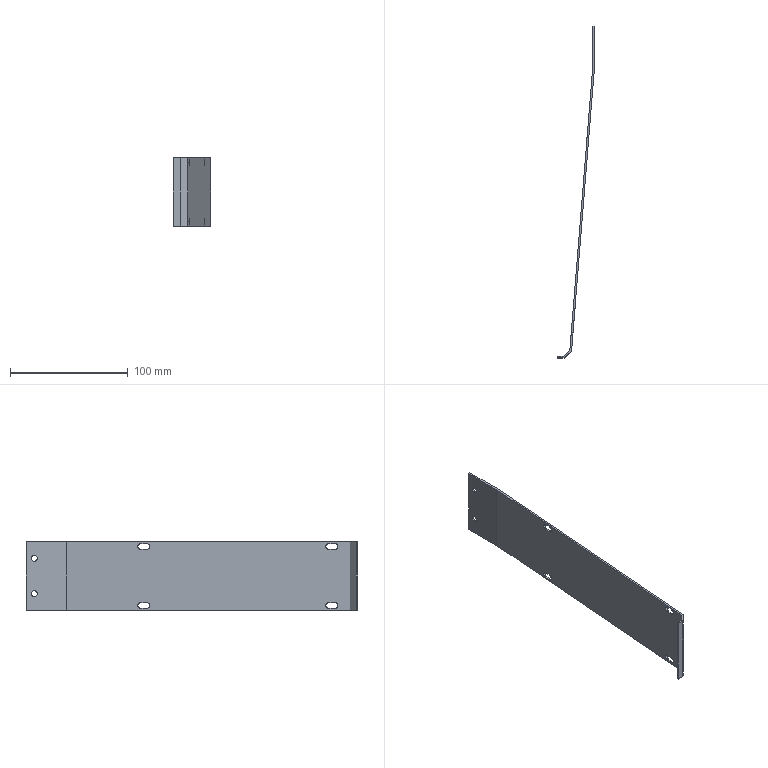Part | SolidWorks | features ICE 2, ExtruThin 1, MirrorPattern 1 | 1 solid | 36 faces | box 31.5 x 281.5 x 58 mm | volume 24856 mm3 | plane 20 | cylinder 16 | commonest cylinder face diameters 5 x16
STEP:
#1=CARTESIAN_POINT('',(-18.024,-256.762,6.5));
#2=VERTEX_POINT('',#1);
#3=CARTESIAN_POINT('',(-17.823,-254.27,4.));
#4=VERTEX_POINT('',#3);
#5=CARTESIAN_POINT('',(-18.024,-256.762,4.));
#6=DIRECTION('',(-0.9967,0.08065,0.));
#7=DIRECTION('',(0.08065,0.9967,0.));
#8=AXIS2_PLACEMENT_3D('',#5,#6,#7);
#9=CIRCLE('',#8,2.5);
#10=EDGE_CURVE('',#2,#4,#9,.T.);
#11=ORIENTED_EDGE('',*,*,#10,.T.);
#12=CARTESIAN_POINT('',(-16.328,-254.391,4.));
#13=VERTEX_POINT('',#12);
#14=CARTESIAN_POINT('',(-26.295,-253.584,4.));
#15=DIRECTION('',(0.9967,-0.08065,0.));
#16=VECTOR('',#15,1000.);
#17=LINE('',#14,#16);
#18=EDGE_CURVE('',#4,#13,#17,.T.);
#19=ORIENTED_EDGE('',*,*,#18,.T.);
#20=CARTESIAN_POINT('',(-16.529,-256.883,6.5));
#21=VERTEX_POINT('',#20);
#22=CARTESIAN_POINT('',(-16.529,-256.883,4.));
#23=DIRECTION('',(-0.9967,0.08065,0.));
#24=DIRECTION('',(-0.08065,-0.9967,0.));
#25=AXIS2_PLACEMENT_3D('',#22,#23,#24);
#26=CIRCLE('',#25,2.5);
#27=EDGE_CURVE('',#21,#13,#26,.T.);
#28=ORIENTED_EDGE('',*,*,#27,.F.);
#29=CARTESIAN_POINT('',(-26.497,-256.076,6.5));
#30=DIRECTION('',(0.9967,-0.08065,0.));
#31=VECTOR('',#30,1000.);
#32=LINE('',#29,#31);
#33=EDGE_CURVE('',#2,#21,#32,.T.);
#34=ORIENTED_EDGE('',*,*,#33,.F.);
#35=EDGE_LOOP('',(#11,#19,#28,#34));
#36=FACE_OUTER_BOUND('',#35,.T.);
#37=CARTESIAN_POINT('',(-26.497,-256.076,4.));
#38=DIRECTION('',(0.9967,-0.08065,0.));
#39=DIRECTION('',(0.08065,0.9967,0.));
#40=AXIS2_PLACEMENT_3D('',#37,#38,#39);
#41=CYLINDRICAL_SURFACE('',#40,2.5);
#42=ADVANCED_FACE('',(#36),#41,.F.);
#43=CARTESIAN_POINT('',(-5.12,-97.283,6.5));
#44=VERTEX_POINT('',#43);
#45=CARTESIAN_POINT('',(-4.919,-94.791,4.));
#46=VERTEX_POINT('',#45);
#47=CARTESIAN_POINT('',(-5.12,-97.283,4.));
#48=DIRECTION('',(-0.9967,0.08065,0.));
#49=DIRECTION('',(0.08065,0.9967,0.));
#50=AXIS2_PLACEMENT_3D('',#47,#48,#49);
#51=CIRCLE('',#50,2.5);
#52=EDGE_CURVE('',#44,#46,#51,.T.);
#53=ORIENTED_EDGE('',*,*,#52,.T.);
#54=CARTESIAN_POINT('',(-3.424,-94.912,4.));
#55=VERTEX_POINT('',#54);
#56=CARTESIAN_POINT('',(-13.391,-94.106,4.));
#57=DIRECTION('',(0.9967,-0.08065,0.));
#58=VECTOR('',#57,1000.);
#59=LINE('',#56,#58);
#60=EDGE_CURVE('',#46,#55,#59,.T.);
#61=ORIENTED_EDGE('',*,*,#60,.T.);
#62=CARTESIAN_POINT('',(-3.625,-97.404,6.5));
#63=VERTEX_POINT('',#62);
#64=CARTESIAN_POINT('',(-3.625,-97.404,4.));
#65=DIRECTION('',(-0.9967,0.08065,0.));
#66=DIRECTION('',(0.08065,0.9967,0.));
#67=AXIS2_PLACEMENT_3D('',#64,#65,#66);
#68=CIRCLE('',#67,2.5);
#69=EDGE_CURVE('',#63,#55,#68,.T.);
#70=ORIENTED_EDGE('',*,*,#69,.F.);
#71=CARTESIAN_POINT('',(-13.593,-96.597,6.5));
#72=DIRECTION('',(0.9967,-0.08065,0.));
#73=VECTOR('',#72,1000.);
#74=LINE('',#71,#73);
#75=EDGE_CURVE('',#44,#63,#74,.T.);
#76=ORIENTED_EDGE('',*,*,#75,.F.);
#77=EDGE_LOOP('',(#53,#61,#70,#76));
#78=FACE_OUTER_BOUND('',#77,.T.);
#79=CARTESIAN_POINT('',(-13.593,-96.597,4.));
#80=DIRECTION('',(0.9967,-0.08065,0.));
#81=DIRECTION('',(0.08065,0.9967,0.));
#82=AXIS2_PLACEMENT_3D('',#79,#80,#81);
#83=CYLINDRICAL_SURFACE('',#82,2.5);
#84=ADVANCED_FACE('',(#78),#83,.F.);
#85=CARTESIAN_POINT('',(-17.823,-254.27,54.));
#86=VERTEX_POINT('',#85);
#87=CARTESIAN_POINT('',(-18.024,-256.762,56.5));
#88=VERTEX_POINT('',#87);
#89=CARTESIAN_POINT('',(-18.024,-256.762,54.));
#90=DIRECTION('',(0.9967,-0.08065,0.));
#91=DIRECTION('',(0.08065,0.9967,0.));
#92=AXIS2_PLACEMENT_3D('',#89,#90,#91);
#93=CIRCLE('',#92,2.5);
#94=EDGE_CURVE('',#86,#88,#93,.T.);
#95=ORIENTED_EDGE('',*,*,#94,.F.);
#96=CARTESIAN_POINT('',(-16.328,-254.391,54.));
#97=VERTEX_POINT('',#96);
#98=CARTESIAN_POINT('',(-26.295,-253.584,54.));
#99=DIRECTION('',(0.9967,-0.08065,0.));
#100=VECTOR('',#99,1000.);
#101=LINE('',#98,#100);
#102=EDGE_CURVE('',#86,#97,#101,.T.);
#103=ORIENTED_EDGE('',*,*,#102,.T.);
#104=CARTESIAN_POINT('',(-16.529,-256.883,56.5));
#105=VERTEX_POINT('',#104);
#106=CARTESIAN_POINT('',(-16.529,-256.883,54.));
#107=DIRECTION('',(0.9967,-0.08065,0.));
#108=DIRECTION('',(-0.08065,-0.9967,0.));
#109=AXIS2_PLACEMENT_3D('',#106,#107,#108);
#110=CIRCLE('',#109,2.5);
#111=EDGE_CURVE('',#97,#105,#110,.T.);
#112=ORIENTED_EDGE('',*,*,#111,.T.);
#113=CARTESIAN_POINT('',(-26.497,-256.076,56.5));
#114=DIRECTION('',(0.9967,-0.08065,0.));
#115=VECTOR('',#114,1000.);
#116=LINE('',#113,#115);
#117=EDGE_CURVE('',#88,#105,#116,.T.);
#118=ORIENTED_EDGE('',*,*,#117,.F.);
#119=EDGE_LOOP('',(#95,#103,#112,#118));
#120=FACE_OUTER_BOUND('',#119,.T.);
#121=CARTESIAN_POINT('',(-26.497,-256.076,54.));
#122=DIRECTION('',(0.9967,-0.08065,0.));
#123=DIRECTION('',(0.08065,0.9967,0.));
#124=AXIS2_PLACEMENT_3D('',#121,#122,#123);
#125=CYLINDRICAL_SURFACE('',#124,2.5);
#126=ADVANCED_FACE('',(#120),#125,.F.);
#127=CARTESIAN_POINT('',(-4.919,-94.791,54.));
#128=VERTEX_POINT('',#127);
#129=CARTESIAN_POINT('',(-5.12,-97.283,56.5));
#130=VERTEX_POINT('',#129);
#131=CARTESIAN_POINT('',(-5.12,-97.283,54.));
#132=DIRECTION('',(0.9967,-0.08065,0.));
#133=DIRECTION('',(0.08065,0.9967,0.));
#134=AXIS2_PLACEMENT_3D('',#131,#132,#133);
#135=CIRCLE('',#134,2.5);
#136=EDGE_CURVE('',#128,#130,#135,.T.);
#137=ORIENTED_EDGE('',*,*,#136,.F.);
#138=CARTESIAN_POINT('',(-3.424,-94.912,54.));
#139=VERTEX_POINT('',#138);
#140=CARTESIAN_POINT('',(-13.391,-94.106,54.));
#141=DIRECTION('',(0.9967,-0.08065,0.));
#142=VECTOR('',#141,1000.);
#143=LINE('',#140,#142);
#144=EDGE_CURVE('',#128,#139,#143,.T.);
#145=ORIENTED_EDGE('',*,*,#144,.T.);
#146=CARTESIAN_POINT('',(-3.625,-97.404,56.5));
#147=VERTEX_POINT('',#146);
#148=CARTESIAN_POINT('',(-3.625,-97.404,54.));
#149=DIRECTION('',(0.9967,-0.08065,0.));
#150=DIRECTION('',(0.08065,0.9967,0.));
#151=AXIS2_PLACEMENT_3D('',#148,#149,#150);
#152=CIRCLE('',#151,2.5);
#153=EDGE_CURVE('',#139,#147,#152,.T.);
#154=ORIENTED_EDGE('',*,*,#153,.T.);
#155=CARTESIAN_POINT('',(-13.593,-96.597,56.5));
#156=DIRECTION('',(0.9967,-0.08065,0.));
#157=VECTOR('',#156,1000.);
#158=LINE('',#155,#157);
#159=EDGE_CURVE('',#130,#147,#158,.T.);
#160=ORIENTED_EDGE('',*,*,#159,.F.);
#161=EDGE_LOOP('',(#137,#145,#154,#160));
#162=FACE_OUTER_BOUND('',#161,.T.);
#163=CARTESIAN_POINT('',(-13.593,-96.597,54.));
#164=DIRECTION('',(0.9967,-0.08065,0.));
#165=DIRECTION('',(0.08065,0.9967,0.));
#166=AXIS2_PLACEMENT_3D('',#163,#164,#165);
#167=CYLINDRICAL_SURFACE('',#166,2.5);
#168=ADVANCED_FACE('',(#162),#167,.F.);
#169=CARTESIAN_POINT('',(0.,-9.5,44.));
#170=VERTEX_POINT('',#169);
#171=CARTESIAN_POINT('',(0.,-4.5,44.));
#172=VERTEX_POINT('',#171);
#173=CARTESIAN_POINT('',(0.,-7.,44.));
#174=DIRECTION('',(1.,0.,0.));
#175=DIRECTION('',(0.,1.,0.));
#176=AXIS2_PLACEMENT_3D('',#173,#174,#175);
#177=CIRCLE('',#176,2.5);
#178=EDGE_CURVE('',#170,#172,#177,.T.);
#179=ORIENTED_EDGE('',*,*,#178,.F.);
#180=CARTESIAN_POINT('',(1.5,-9.5,44.));
#181=VERTEX_POINT('',#180);
#182=CARTESIAN_POINT('',(-8.5,-9.5,44.));
#183=DIRECTION('',(1.,0.,0.));
#184=VECTOR('',#183,1000.);
#185=LINE('',#182,#184);
#186=EDGE_CURVE('',#170,#181,#185,.T.);
#187=ORIENTED_EDGE('',*,*,#186,.T.);
#188=CARTESIAN_POINT('',(1.5,-4.5,44.));
#189=VERTEX_POINT('',#188);
#190=CARTESIAN_POINT('',(1.5,-7.,44.));
#191=DIRECTION('',(1.,0.,0.));
#192=DIRECTION('',(0.,1.,0.));
#193=AXIS2_PLACEMENT_3D('',#190,#191,#192);
#194=CIRCLE('',#193,2.5);
#195=EDGE_CURVE('',#181,#189,#194,.T.);
#196=ORIENTED_EDGE('',*,*,#195,.T.);
#197=CARTESIAN_POINT('',(-8.5,-4.5,44.));
#198=DIRECTION('',(1.,0.,0.));
#199=VECTOR('',#198,1000.);
#200=LINE('',#197,#199);
#201=EDGE_CURVE('',#172,#189,#200,.T.);
#202=ORIENTED_EDGE('',*,*,#201,.F.);
#203=EDGE_LOOP('',(#179,#187,#196,#202));
#204=FACE_OUTER_BOUND('',#203,.T.);
#205=CARTESIAN_POINT('',(-8.5,-7.,44.));
#206=DIRECTION('',(1.,0.,0.));
#207=DIRECTION('',(0.,1.,0.));
#208=AXIS2_PLACEMENT_3D('',#205,#206,#207);
#209=CYLINDRICAL_SURFACE('',#208,2.5);
#210=ADVANCED_FACE('',(#204),#209,.F.);
#211=CARTESIAN_POINT('',(0.,-9.5,14.));
#212=VERTEX_POINT('',#211);
#213=CARTESIAN_POINT('',(0.,-4.5,14.));
#214=VERTEX_POINT('',#213);
#215=CARTESIAN_POINT('',(0.,-7.,14.));
#216=DIRECTION('',(1.,0.,0.));
#217=DIRECTION('',(0.,1.,0.));
#218=AXIS2_PLACEMENT_3D('',#215,#216,#217);
#219=CIRCLE('',#218,2.5);
#220=EDGE_CURVE('',#212,#214,#219,.T.);
#221=ORIENTED_EDGE('',*,*,#220,.F.);
#222=CARTESIAN_POINT('',(1.5,-9.5,14.));
#223=VERTEX_POINT('',#222);
#224=CARTESIAN_POINT('',(-8.5,-9.5,14.));
#225=DIRECTION('',(1.,0.,0.));
#226=VECTOR('',#225,1000.);
#227=LINE('',#224,#226);
#228=EDGE_CURVE('',#212,#223,#227,.T.);
#229=ORIENTED_EDGE('',*,*,#228,.T.);
#230=CARTESIAN_POINT('',(1.5,-4.5,14.));
#231=VERTEX_POINT('',#230);
#232=CARTESIAN_POINT('',(1.5,-7.,14.));
#233=DIRECTION('',(1.,0.,0.));
#234=DIRECTION('',(0.,1.,0.));
#235=AXIS2_PLACEMENT_3D('',#232,#233,#234);
#236=CIRCLE('',#235,2.5);
#237=EDGE_CURVE('',#223,#231,#236,.T.);
#238=ORIENTED_EDGE('',*,*,#237,.T.);
#239=CARTESIAN_POINT('',(-8.5,-4.5,14.));
#240=DIRECTION('',(1.,0.,0.));
#241=VECTOR('',#240,1000.);
#242=LINE('',#239,#241);
#243=EDGE_CURVE('',#214,#231,#242,.T.);
#244=ORIENTED_EDGE('',*,*,#243,.F.);
#245=EDGE_LOOP('',(#221,#229,#238,#244));
#246=FACE_OUTER_BOUND('',#245,.T.);
#247=CARTESIAN_POINT('',(-8.5,-7.,14.));
#248=DIRECTION('',(1.,0.,0.));
#249=DIRECTION('',(0.,1.,0.));
#250=AXIS2_PLACEMENT_3D('',#247,#248,#249);
#251=CYLINDRICAL_SURFACE('',#250,2.5);
#252=ADVANCED_FACE('',(#246),#251,.F.);
#253=CARTESIAN_POINT('',(-4.029,-102.388,6.5));
#254=VERTEX_POINT('',#253);
#255=CARTESIAN_POINT('',(-3.625,-97.404,6.5));
#256=DIRECTION('',(0.08065,0.9967,0.));
#257=VECTOR('',#256,1000.);
#258=LINE('',#255,#257);
#259=EDGE_CURVE('',#254,#63,#258,.T.);
#260=ORIENTED_EDGE('',*,*,#259,.T.);
#261=ORIENTED_EDGE('',*,*,#69,.T.);
#262=CARTESIAN_POINT('',(-3.625,-97.404,1.5));
#263=VERTEX_POINT('',#262);
#264=CARTESIAN_POINT('',(-3.625,-97.404,4.));
#265=DIRECTION('',(-0.9967,0.08065,0.));
#266=DIRECTION('',(0.08065,0.9967,0.));
#267=AXIS2_PLACEMENT_3D('',#264,#265,#266);
#268=CIRCLE('',#267,2.5);
#269=EDGE_CURVE('',#55,#263,#268,.T.);
#270=ORIENTED_EDGE('',*,*,#269,.T.);
#271=CARTESIAN_POINT('',(-4.029,-102.388,1.5));
#272=VERTEX_POINT('',#271);
#273=CARTESIAN_POINT('',(-3.625,-97.404,1.5));
#274=DIRECTION('',(-0.08065,-0.9967,0.));
#275=VECTOR('',#274,1000.);
#276=LINE('',#273,#275);
#277=EDGE_CURVE('',#263,#272,#276,.T.);
#278=ORIENTED_EDGE('',*,*,#277,.T.);
#279=CARTESIAN_POINT('',(-4.029,-102.388,4.));
#280=DIRECTION('',(-0.9967,0.08065,0.));
#281=DIRECTION('',(0.08065,0.9967,0.));
#282=AXIS2_PLACEMENT_3D('',#279,#280,#281);
#283=CIRCLE('',#282,2.5);
#284=EDGE_CURVE('',#272,#254,#283,.T.);
#285=ORIENTED_EDGE('',*,*,#284,.T.);
#286=EDGE_LOOP('',(#260,#261,#270,#278,#285));
#287=FACE_BOUND('',#286,.T.);
#288=CARTESIAN_POINT('',(-16.932,-261.866,56.5));
#289=VERTEX_POINT('',#288);
#290=CARTESIAN_POINT('',(-16.932,-261.866,51.5));
#291=VERTEX_POINT('',#290);
#292=CARTESIAN_POINT('',(-16.932,-261.866,54.));
#293=DIRECTION('',(0.9967,-0.08065,0.));
#294=DIRECTION('',(-0.08065,-0.9967,0.));
#295=AXIS2_PLACEMENT_3D('',#292,#293,#294);
#296=CIRCLE('',#295,2.5);
#297=EDGE_CURVE('',#289,#291,#296,.T.);
#298=ORIENTED_EDGE('',*,*,#297,.F.);
#299=CARTESIAN_POINT('',(-16.932,-261.866,56.5));
#300=DIRECTION('',(-0.08065,-0.9967,0.));
#301=VECTOR('',#300,1000.);
#302=LINE('',#299,#301);
#303=EDGE_CURVE('',#105,#289,#302,.T.);
#304=ORIENTED_EDGE('',*,*,#303,.F.);
#305=ORIENTED_EDGE('',*,*,#111,.F.);
#306=CARTESIAN_POINT('',(-16.529,-256.883,51.5));
#307=VERTEX_POINT('',#306);
#308=CARTESIAN_POINT('',(-16.529,-256.883,54.));
#309=DIRECTION('',(0.9967,-0.08065,0.));
#310=DIRECTION('',(-0.08065,-0.9967,0.));
#311=AXIS2_PLACEMENT_3D('',#308,#309,#310);
#312=CIRCLE('',#311,2.5);
#313=EDGE_CURVE('',#307,#97,#312,.T.);
#314=ORIENTED_EDGE('',*,*,#313,.F.);
#315=CARTESIAN_POINT('',(-16.932,-261.866,51.5));
#316=DIRECTION('',(0.08065,0.9967,0.));
#317=VECTOR('',#316,1000.);
#318=LINE('',#315,#317);
#319=EDGE_CURVE('',#291,#307,#318,.T.);
#320=ORIENTED_EDGE('',*,*,#319,.F.);
#321=EDGE_LOOP('',(#298,#304,#305,#314,#320));
#322=FACE_BOUND('',#321,.T.);
#323=CARTESIAN_POINT('',(-3.625,-97.404,51.5));
#324=VERTEX_POINT('',#323);
#325=CARTESIAN_POINT('',(-3.625,-97.404,54.));
#326=DIRECTION('',(0.9967,-0.08065,0.));
#327=DIRECTION('',(0.08065,0.9967,0.));
#328=AXIS2_PLACEMENT_3D('',#325,#326,#327);
#329=CIRCLE('',#328,2.5);
#330=EDGE_CURVE('',#324,#139,#329,.T.);
#331=ORIENTED_EDGE('',*,*,#330,.F.);
#332=CARTESIAN_POINT('',(-4.029,-102.388,51.5));
#333=VERTEX_POINT('',#332);
#334=CARTESIAN_POINT('',(-3.625,-97.404,51.5));
#335=DIRECTION('',(0.08065,0.9967,0.));
#336=VECTOR('',#335,1000.);
#337=LINE('',#334,#336);
#338=EDGE_CURVE('',#333,#324,#337,.T.);
#339=ORIENTED_EDGE('',*,*,#338,.F.);
#340=CARTESIAN_POINT('',(-4.029,-102.388,56.5));
#341=VERTEX_POINT('',#340);
#342=CARTESIAN_POINT('',(-4.029,-102.388,54.));
#343=DIRECTION('',(0.9967,-0.08065,0.));
#344=DIRECTION('',(0.08065,0.9967,0.));
#345=AXIS2_PLACEMENT_3D('',#342,#343,#344);
#346=CIRCLE('',#345,2.5);
#347=EDGE_CURVE('',#341,#333,#346,.T.);
#348=ORIENTED_EDGE('',*,*,#347,.F.);
#349=CARTESIAN_POINT('',(-3.625,-97.404,56.5));
#350=DIRECTION('',(-0.08065,-0.9967,0.));
#351=VECTOR('',#350,1000.);
#352=LINE('',#349,#351);
#353=EDGE_CURVE('',#147,#341,#352,.T.);
#354=ORIENTED_EDGE('',*,*,#353,.F.);
#355=ORIENTED_EDGE('',*,*,#153,.F.);
#356=EDGE_LOOP('',(#331,#339,#348,#354,#355));
#357=FACE_BOUND('',#356,.T.);
#358=CARTESIAN_POINT('',(1.5,-34.061,0.));
#359=VERTEX_POINT('',#358);
#360=CARTESIAN_POINT('',(-18.053,-275.711,0.));
#361=VERTEX_POINT('',#360);
#362=CARTESIAN_POINT('',(1.495,-34.121,0.));
#363=DIRECTION('',(-0.08065,-0.9967,0.));
#364=VECTOR('',#363,1000.);
#365=LINE('',#362,#364);
#366=EDGE_CURVE('',#359,#361,#365,.T.);
#367=ORIENTED_EDGE('',*,*,#366,.F.);
#368=CARTESIAN_POINT('',(1.5,-34.061,58.));
#369=VERTEX_POINT('',#368);
#370=CARTESIAN_POINT('',(1.5,-34.061,58.));
#371=DIRECTION('',(0.,0.,-1.));
#372=VECTOR('',#371,1000.);
#373=LINE('',#370,#372);
#374=EDGE_CURVE('',#369,#359,#373,.T.);
#375=ORIENTED_EDGE('',*,*,#374,.F.);
#376=CARTESIAN_POINT('',(-18.053,-275.711,58.));
#377=VERTEX_POINT('',#376);
#378=CARTESIAN_POINT('',(1.495,-34.121,58.));
#379=DIRECTION('',(-0.08065,-0.9967,0.));
#380=VECTOR('',#379,1000.);
#381=LINE('',#378,#380);
#382=EDGE_CURVE('',#369,#377,#381,.T.);
#383=ORIENTED_EDGE('',*,*,#382,.T.);
#384=CARTESIAN_POINT('',(-18.053,-275.711,58.));
#385=DIRECTION('',(0.,0.,-1.));
#386=VECTOR('',#385,1000.);
#387=LINE('',#384,#386);
#388=EDGE_CURVE('',#377,#361,#387,.T.);
#389=ORIENTED_EDGE('',*,*,#388,.T.);
#390=EDGE_LOOP('',(#367,#375,#383,#389));
#391=FACE_OUTER_BOUND('',#390,.T.);
#392=CARTESIAN_POINT('',(-16.529,-256.883,1.5));
#393=VERTEX_POINT('',#392);
#394=CARTESIAN_POINT('',(-16.932,-261.866,1.5));
#395=VERTEX_POINT('',#394);
#396=CARTESIAN_POINT('',(-16.932,-261.866,1.5));
#397=DIRECTION('',(-0.08065,-0.9967,0.));
#398=VECTOR('',#397,1000.);
#399=LINE('',#396,#398);
#400=EDGE_CURVE('',#393,#395,#399,.T.);
#401=ORIENTED_EDGE('',*,*,#400,.T.);
#402=CARTESIAN_POINT('',(-16.932,-261.866,6.5));
#403=VERTEX_POINT('',#402);
#404=CARTESIAN_POINT('',(-16.932,-261.866,4.));
#405=DIRECTION('',(-0.9967,0.08065,0.));
#406=DIRECTION('',(-0.08065,-0.9967,0.));
#407=AXIS2_PLACEMENT_3D('',#404,#405,#406);
#408=CIRCLE('',#407,2.5);
#409=EDGE_CURVE('',#395,#403,#408,.T.);
#410=ORIENTED_EDGE('',*,*,#409,.T.);
#411=CARTESIAN_POINT('',(-16.932,-261.866,6.5));
#412=DIRECTION('',(0.08065,0.9967,0.));
#413=VECTOR('',#412,1000.);
#414=LINE('',#411,#413);
#415=EDGE_CURVE('',#403,#21,#414,.T.);
#416=ORIENTED_EDGE('',*,*,#415,.T.);
#417=ORIENTED_EDGE('',*,*,#27,.T.);
#418=CARTESIAN_POINT('',(-16.529,-256.883,4.));
#419=DIRECTION('',(-0.9967,0.08065,0.));
#420=DIRECTION('',(-0.08065,-0.9967,0.));
#421=AXIS2_PLACEMENT_3D('',#418,#419,#420);
#422=CIRCLE('',#421,2.5);
#423=EDGE_CURVE('',#13,#393,#422,.T.);
#424=ORIENTED_EDGE('',*,*,#423,.T.);
#425=EDGE_LOOP('',(#401,#410,#416,#417,#424));
#426=FACE_BOUND('',#425,.T.);
#427=CARTESIAN_POINT('',(1.495,-34.121,58.));
#428=DIRECTION('',(0.9967,-0.08065,0.));
#429=DIRECTION('',(0.08065,0.9967,0.));
#430=AXIS2_PLACEMENT_3D('',#427,#428,#429);
#431=PLANE('',#430);
#432=ADVANCED_FACE('',(#287,#322,#357,#391,#426),#431,.T.);
#433=ORIENTED_EDGE('',*,*,#52,.F.);
#434=CARTESIAN_POINT('',(-5.524,-102.267,6.5));
#435=VERTEX_POINT('',#434);
#436=CARTESIAN_POINT('',(0.,-34.,6.5));
#437=DIRECTION('',(0.08065,0.9967,0.));
#438=VECTOR('',#437,1000.);
#439=LINE('',#436,#438);
#440=EDGE_CURVE('',#435,#44,#439,.T.);
#441=ORIENTED_EDGE('',*,*,#440,.F.);
#442=CARTESIAN_POINT('',(-5.524,-102.267,1.5));
#443=VERTEX_POINT('',#442);
#444=CARTESIAN_POINT('',(-5.524,-102.267,4.));
#445=DIRECTION('',(-0.9967,0.08065,0.));
#446=DIRECTION('',(0.08065,0.9967,0.));
#447=AXIS2_PLACEMENT_3D('',#444,#445,#446);
#448=CIRCLE('',#447,2.5);
#449=EDGE_CURVE('',#443,#435,#448,.T.);
#450=ORIENTED_EDGE('',*,*,#449,.F.);
#451=CARTESIAN_POINT('',(-5.12,-97.283,1.5));
#452=VERTEX_POINT('',#451);
#453=CARTESIAN_POINT('',(0.,-34.,1.5));
#454=DIRECTION('',(-0.08065,-0.9967,0.));
#455=VECTOR('',#454,1000.);
#456=LINE('',#453,#455);
#457=EDGE_CURVE('',#452,#443,#456,.T.);
#458=ORIENTED_EDGE('',*,*,#457,.F.);
#459=CARTESIAN_POINT('',(-5.12,-97.283,4.));
#460=DIRECTION('',(-0.9967,0.08065,0.));
#461=DIRECTION('',(0.08065,0.9967,0.));
#462=AXIS2_PLACEMENT_3D('',#459,#460,#461);
#463=CIRCLE('',#462,2.5);
#464=EDGE_CURVE('',#46,#452,#463,.T.);
#465=ORIENTED_EDGE('',*,*,#464,.F.);
#466=EDGE_LOOP('',(#433,#441,#450,#458,#465));
#467=FACE_BOUND('',#466,.T.);
#468=CARTESIAN_POINT('',(-18.428,-261.745,56.5));
#469=VERTEX_POINT('',#468);
#470=CARTESIAN_POINT('',(0.,-34.,56.5));
#471=DIRECTION('',(-0.08065,-0.9967,0.));
#472=VECTOR('',#471,1000.);
#473=LINE('',#470,#472);
#474=EDGE_CURVE('',#88,#469,#473,.T.);
#475=ORIENTED_EDGE('',*,*,#474,.T.);
#476=CARTESIAN_POINT('',(-18.428,-261.745,51.5));
#477=VERTEX_POINT('',#476);
#478=CARTESIAN_POINT('',(-18.428,-261.745,54.));
#479=DIRECTION('',(0.9967,-0.08065,0.));
#480=DIRECTION('',(0.08065,0.9967,0.));
#481=AXIS2_PLACEMENT_3D('',#478,#479,#480);
#482=CIRCLE('',#481,2.5);
#483=EDGE_CURVE('',#469,#477,#482,.T.);
#484=ORIENTED_EDGE('',*,*,#483,.T.);
#485=CARTESIAN_POINT('',(-18.024,-256.762,51.5));
#486=VERTEX_POINT('',#485);
#487=CARTESIAN_POINT('',(0.,-34.,51.5));
#488=DIRECTION('',(0.08065,0.9967,0.));
#489=VECTOR('',#488,1000.);
#490=LINE('',#487,#489);
#491=EDGE_CURVE('',#477,#486,#490,.T.);
#492=ORIENTED_EDGE('',*,*,#491,.T.);
#493=CARTESIAN_POINT('',(-18.024,-256.762,54.));
#494=DIRECTION('',(0.9967,-0.08065,0.));
#495=DIRECTION('',(0.08065,0.9967,0.));
#496=AXIS2_PLACEMENT_3D('',#493,#494,#495);
#497=CIRCLE('',#496,2.5);
#498=EDGE_CURVE('',#486,#86,#497,.T.);
#499=ORIENTED_EDGE('',*,*,#498,.T.);
#500=ORIENTED_EDGE('',*,*,#94,.T.);
#501=EDGE_LOOP('',(#475,#484,#492,#499,#500));
#502=FACE_BOUND('',#501,.T.);
#503=CARTESIAN_POINT('',(-5.524,-102.267,51.5));
#504=VERTEX_POINT('',#503);
#505=CARTESIAN_POINT('',(-5.12,-97.283,51.5));
#506=VERTEX_POINT('',#505);
#507=CARTESIAN_POINT('',(0.,-34.,51.5));
#508=DIRECTION('',(0.08065,0.9967,0.));
#509=VECTOR('',#508,1000.);
#510=LINE('',#507,#509);
#511=EDGE_CURVE('',#504,#506,#510,.T.);
#512=ORIENTED_EDGE('',*,*,#511,.T.);
#513=CARTESIAN_POINT('',(-5.12,-97.283,54.));
#514=DIRECTION('',(0.9967,-0.08065,0.));
#515=DIRECTION('',(0.08065,0.9967,0.));
#516=AXIS2_PLACEMENT_3D('',#513,#514,#515);
#517=CIRCLE('',#516,2.5);
#518=EDGE_CURVE('',#506,#128,#517,.T.);
#519=ORIENTED_EDGE('',*,*,#518,.T.);
#520=ORIENTED_EDGE('',*,*,#136,.T.);
#521=CARTESIAN_POINT('',(-5.524,-102.267,56.5));
#522=VERTEX_POINT('',#521);
#523=CARTESIAN_POINT('',(0.,-34.,56.5));
#524=DIRECTION('',(-0.08065,-0.9967,0.));
#525=VECTOR('',#524,1000.);
#526=LINE('',#523,#525);
#527=EDGE_CURVE('',#130,#522,#526,.T.);
#528=ORIENTED_EDGE('',*,*,#527,.T.);
#529=CARTESIAN_POINT('',(-5.524,-102.267,54.));
#530=DIRECTION('',(0.9967,-0.08065,0.));
#531=DIRECTION('',(0.08065,0.9967,0.));
#532=AXIS2_PLACEMENT_3D('',#529,#530,#531);
#533=CIRCLE('',#532,2.5);
#534=EDGE_CURVE('',#522,#504,#533,.T.);
#535=ORIENTED_EDGE('',*,*,#534,.T.);
#536=EDGE_LOOP('',(#512,#519,#520,#528,#535));
#537=FACE_BOUND('',#536,.T.);
#538=CARTESIAN_POINT('',(0.,-34.,0.));
#539=VERTEX_POINT('',#538);
#540=CARTESIAN_POINT('',(-19.5,-275.,0.));
#541=VERTEX_POINT('',#540);
#542=CARTESIAN_POINT('',(0.,-34.,0.));
#543=DIRECTION('',(-0.08065,-0.9967,0.));
#544=VECTOR('',#543,1000.);
#545=LINE('',#542,#544);
#546=EDGE_CURVE('',#539,#541,#545,.T.);
#547=ORIENTED_EDGE('',*,*,#546,.T.);
#548=CARTESIAN_POINT('',(-19.5,-275.,58.));
#549=VERTEX_POINT('',#548);
#550=CARTESIAN_POINT('',(-19.5,-275.,58.));
#551=DIRECTION('',(0.,0.,-1.));
#552=VECTOR('',#551,1000.);
#553=LINE('',#550,#552);
#554=EDGE_CURVE('',#549,#541,#553,.T.);
#555=ORIENTED_EDGE('',*,*,#554,.F.);
#556=CARTESIAN_POINT('',(0.,-34.,58.));
#557=VERTEX_POINT('',#556);
#558=CARTESIAN_POINT('',(0.,-34.,58.));
#559=DIRECTION('',(-0.08065,-0.9967,0.));
#560=VECTOR('',#559,1000.);
#561=LINE('',#558,#560);
#562=EDGE_CURVE('',#557,#549,#561,.T.);
#563=ORIENTED_EDGE('',*,*,#562,.F.);
#564=CARTESIAN_POINT('',(0.,-34.,58.));
#565=DIRECTION('',(0.,0.,-1.));
#566=VECTOR('',#565,1000.);
#567=LINE('',#564,#566);
#568=EDGE_CURVE('',#557,#539,#567,.T.);
#569=ORIENTED_EDGE('',*,*,#568,.T.);
#570=EDGE_LOOP('',(#547,#555,#563,#569));
#571=FACE_OUTER_BOUND('',#570,.T.);
#572=CARTESIAN_POINT('',(-18.428,-261.745,1.5));
#573=VERTEX_POINT('',#572);
#574=CARTESIAN_POINT('',(-18.428,-261.745,6.5));
#575=VERTEX_POINT('',#574);
#576=CARTESIAN_POINT('',(-18.428,-261.745,4.));
#577=DIRECTION('',(-0.9967,0.08065,0.));
#578=DIRECTION('',(0.08065,0.9967,0.));
#579=AXIS2_PLACEMENT_3D('',#576,#577,#578);
#580=CIRCLE('',#579,2.5);
#581=EDGE_CURVE('',#573,#575,#580,.T.);
#582=ORIENTED_EDGE('',*,*,#581,.F.);
#583=CARTESIAN_POINT('',(-18.024,-256.762,1.5));
#584=VERTEX_POINT('',#583);
#585=CARTESIAN_POINT('',(0.,-34.,1.5));
#586=DIRECTION('',(-0.08065,-0.9967,0.));
#587=VECTOR('',#586,1000.);
#588=LINE('',#585,#587);
#589=EDGE_CURVE('',#584,#573,#588,.T.);
#590=ORIENTED_EDGE('',*,*,#589,.F.);
#591=CARTESIAN_POINT('',(-18.024,-256.762,4.));
#592=DIRECTION('',(-0.9967,0.08065,0.));
#593=DIRECTION('',(0.08065,0.9967,0.));
#594=AXIS2_PLACEMENT_3D('',#591,#592,#593);
#595=CIRCLE('',#594,2.5);
#596=EDGE_CURVE('',#4,#584,#595,.T.);
#597=ORIENTED_EDGE('',*,*,#596,.F.);
#598=ORIENTED_EDGE('',*,*,#10,.F.);
#599=CARTESIAN_POINT('',(0.,-34.,6.5));
#600=DIRECTION('',(0.08065,0.9967,0.));
#601=VECTOR('',#600,1000.);
#602=LINE('',#599,#601);
#603=EDGE_CURVE('',#575,#2,#602,.T.);
#604=ORIENTED_EDGE('',*,*,#603,.F.);
#605=EDGE_LOOP('',(#582,#590,#597,#598,#604));
#606=FACE_BOUND('',#605,.T.);
#607=CARTESIAN_POINT('',(0.,-34.,58.));
#608=DIRECTION('',(0.9967,-0.08065,0.));
#609=DIRECTION('',(0.08065,0.9967,0.));
#610=AXIS2_PLACEMENT_3D('',#607,#608,#609);
#611=PLANE('',#610);
#612=ADVANCED_FACE('',(#467,#502,#537,#571,#606),#611,.F.);
#613=CARTESIAN_POINT('',(-25.,-280.,0.));
#614=VERTEX_POINT('',#613);
#615=CARTESIAN_POINT('',(-30.,-280.,0.));
#616=VERTEX_POINT('',#615);
#617=CARTESIAN_POINT('',(-25.,-280.,0.));
#618=DIRECTION('',(-1.,0.,0.));
#619=VECTOR('',#618,1000.);
#620=LINE('',#617,#619);
#621=EDGE_CURVE('',#614,#616,#620,.T.);
#622=ORIENTED_EDGE('',*,*,#621,.T.);
#623=CARTESIAN_POINT('',(-30.,-280.,58.));
#624=VERTEX_POINT('',#623);
#625=CARTESIAN_POINT('',(-30.,-280.,58.));
#626=DIRECTION('',(0.,0.,-1.));
#627=VECTOR('',#626,1000.);
#628=LINE('',#625,#627);
#629=EDGE_CURVE('',#624,#616,#628,.T.);
#630=ORIENTED_EDGE('',*,*,#629,.F.);
#631=CARTESIAN_POINT('',(-25.,-280.,58.));
#632=VERTEX_POINT('',#631);
#633=CARTESIAN_POINT('',(-25.,-280.,58.));
#634=DIRECTION('',(-1.,0.,0.));
#635=VECTOR('',#634,1000.);
#636=LINE('',#633,#635);
#637=EDGE_CURVE('',#632,#624,#636,.T.);
#638=ORIENTED_EDGE('',*,*,#637,.F.);
#639=CARTESIAN_POINT('',(-25.,-280.,58.));
#640=DIRECTION('',(0.,0.,-1.));
#641=VECTOR('',#640,1000.);
#642=LINE('',#639,#641);
#643=EDGE_CURVE('',#632,#614,#642,.T.);
#644=ORIENTED_EDGE('',*,*,#643,.T.);
#645=EDGE_LOOP('',(#622,#630,#638,#644));
#646=FACE_OUTER_BOUND('',#645,.T.);
#647=CARTESIAN_POINT('',(-25.,-280.,58.));
#648=DIRECTION('',(0.,-1.,0.));
#649=DIRECTION('',(1.,0.,0.));
#650=AXIS2_PLACEMENT_3D('',#647,#648,#649);
#651=PLANE('',#650);
#652=ADVANCED_FACE('',(#646),#651,.F.);
#653=CARTESIAN_POINT('',(-30.,-281.5,0.));
#654=VERTEX_POINT('',#653);
#655=CARTESIAN_POINT('',(-30.,-281.5,0.));
#656=DIRECTION('',(0.,1.,0.));
#657=VECTOR('',#656,1000.);
#658=LINE('',#655,#657);
#659=EDGE_CURVE('',#654,#616,#658,.T.);
#660=ORIENTED_EDGE('',*,*,#659,.F.);
#661=CARTESIAN_POINT('',(-30.,-281.5,58.));
#662=VERTEX_POINT('',#661);
#663=CARTESIAN_POINT('',(-30.,-281.5,58.));
#664=DIRECTION('',(0.,0.,-1.));
#665=VECTOR('',#664,1000.);
#666=LINE('',#663,#665);
#667=EDGE_CURVE('',#662,#654,#666,.T.);
#668=ORIENTED_EDGE('',*,*,#667,.F.);
#669=CARTESIAN_POINT('',(-30.,-281.5,58.));
#670=DIRECTION('',(0.,1.,0.));
#671=VECTOR('',#670,1000.);
#672=LINE('',#669,#671);
#673=EDGE_CURVE('',#662,#624,#672,.T.);
#674=ORIENTED_EDGE('',*,*,#673,.T.);
#675=ORIENTED_EDGE('',*,*,#629,.T.);
#676=EDGE_LOOP('',(#660,#668,#674,#675));
#677=FACE_OUTER_BOUND('',#676,.T.);
#678=CARTESIAN_POINT('',(-30.,-281.5,58.));
#679=DIRECTION('',(-1.,0.,0.));
#680=DIRECTION('',(0.,-1.,0.));
#681=AXIS2_PLACEMENT_3D('',#678,#679,#680);
#682=PLANE('',#681);
#683=ADVANCED_FACE('',(#677),#682,.T.);
#684=CARTESIAN_POINT('',(-24.42,-281.5,0.));
#685=VERTEX_POINT('',#684);
#686=CARTESIAN_POINT('',(-25.,-281.5,0.));
#687=DIRECTION('',(-1.,0.,0.));
#688=VECTOR('',#687,1000.);
#689=LINE('',#686,#688);
#690=EDGE_CURVE('',#685,#654,#689,.T.);
#691=ORIENTED_EDGE('',*,*,#690,.F.);
#692=CARTESIAN_POINT('',(-24.42,-281.5,58.));
#693=VERTEX_POINT('',#692);
#694=CARTESIAN_POINT('',(-24.42,-281.5,58.));
#695=DIRECTION('',(0.,0.,-1.));
#696=VECTOR('',#695,1000.);
#697=LINE('',#694,#696);
#698=EDGE_CURVE('',#693,#685,#697,.T.);
#699=ORIENTED_EDGE('',*,*,#698,.F.);
#700=CARTESIAN_POINT('',(-25.,-281.5,58.));
#701=DIRECTION('',(-1.,0.,0.));
#702=VECTOR('',#701,1000.);
#703=LINE('',#700,#702);
#704=EDGE_CURVE('',#693,#662,#703,.T.);
#705=ORIENTED_EDGE('',*,*,#704,.T.);
#706=ORIENTED_EDGE('',*,*,#667,.T.);
#707=EDGE_LOOP('',(#691,#699,#705,#706));
#708=FACE_OUTER_BOUND('',#707,.T.);
#709=CARTESIAN_POINT('',(-25.,-281.5,58.));
#710=DIRECTION('',(0.,-1.,0.));
#711=DIRECTION('',(1.,0.,0.));
#712=AXIS2_PLACEMENT_3D('',#709,#710,#711);
#713=PLANE('',#712);
#714=ADVANCED_FACE('',(#708),#713,.T.);
#715=CARTESIAN_POINT('',(-18.491,-276.11,0.));
#716=DIRECTION('',(-0.7399,-0.6727,0.));
#717=VECTOR('',#716,1000.);
#718=LINE('',#715,#717);
#719=EDGE_CURVE('',#361,#685,#718,.T.);
#720=ORIENTED_EDGE('',*,*,#719,.F.);
#721=ORIENTED_EDGE('',*,*,#388,.F.);
#722=CARTESIAN_POINT('',(-18.491,-276.11,58.));
#723=DIRECTION('',(-0.7399,-0.6727,0.));
#724=VECTOR('',#723,1000.);
#725=LINE('',#722,#724);
#726=EDGE_CURVE('',#377,#693,#725,.T.);
#727=ORIENTED_EDGE('',*,*,#726,.T.);
#728=ORIENTED_EDGE('',*,*,#698,.T.);
#729=EDGE_LOOP('',(#720,#721,#727,#728));
#730=FACE_OUTER_BOUND('',#729,.T.);
#731=CARTESIAN_POINT('',(-18.491,-276.11,58.));
#732=DIRECTION('',(0.6727,-0.7399,0.));
#733=DIRECTION('',(0.7399,0.6727,0.));
#734=AXIS2_PLACEMENT_3D('',#731,#732,#733);
#735=PLANE('',#734);
#736=ADVANCED_FACE('',(#730),#735,.T.);
#737=CARTESIAN_POINT('',(1.5,-7.,44.));
#738=DIRECTION('',(1.,0.,0.));
#739=DIRECTION('',(0.,1.,0.));
#740=AXIS2_PLACEMENT_3D('',#737,#738,#739);
#741=CIRCLE('',#740,2.5);
#742=EDGE_CURVE('',#189,#181,#741,.T.);
#743=ORIENTED_EDGE('',*,*,#742,.F.);
#744=ORIENTED_EDGE('',*,*,#195,.F.);
#745=EDGE_LOOP('',(#743,#744));
#746=FACE_BOUND('',#745,.T.);
#747=CARTESIAN_POINT('',(1.5,-7.,14.));
#748=DIRECTION('',(1.,0.,0.));
#749=DIRECTION('',(0.,1.,0.));
#750=AXIS2_PLACEMENT_3D('',#747,#748,#749);
#751=CIRCLE('',#750,2.5);
#752=EDGE_CURVE('',#231,#223,#751,.T.);
#753=ORIENTED_EDGE('',*,*,#752,.F.);
#754=ORIENTED_EDGE('',*,*,#237,.F.);
#755=EDGE_LOOP('',(#753,#754));
#756=FACE_BOUND('',#755,.T.);
#757=CARTESIAN_POINT('',(1.5,0.,0.));
#758=VERTEX_POINT('',#757);
#759=CARTESIAN_POINT('',(1.5,0.,0.));
#760=DIRECTION('',(0.,-1.,0.));
#761=VECTOR('',#760,1000.);
#762=LINE('',#759,#761);
#763=EDGE_CURVE('',#758,#359,#762,.T.);
#764=ORIENTED_EDGE('',*,*,#763,.F.);
#765=CARTESIAN_POINT('',(1.5,0.,58.));
#766=VERTEX_POINT('',#765);
#767=CARTESIAN_POINT('',(1.5,0.,58.));
#768=DIRECTION('',(0.,0.,-1.));
#769=VECTOR('',#768,1000.);
#770=LINE('',#767,#769);
#771=EDGE_CURVE('',#766,#758,#770,.T.);
#772=ORIENTED_EDGE('',*,*,#771,.F.);
#773=CARTESIAN_POINT('',(1.5,0.,58.));
#774=DIRECTION('',(0.,-1.,0.));
#775=VECTOR('',#774,1000.);
#776=LINE('',#773,#775);
#777=EDGE_CURVE('',#766,#369,#776,.T.);
#778=ORIENTED_EDGE('',*,*,#777,.T.);
#779=ORIENTED_EDGE('',*,*,#374,.T.);
#780=EDGE_LOOP('',(#764,#772,#778,#779));
#781=FACE_OUTER_BOUND('',#780,.T.);
#782=CARTESIAN_POINT('',(1.5,0.,58.));
#783=DIRECTION('',(1.,0.,0.));
#784=DIRECTION('',(0.,1.,0.));
#785=AXIS2_PLACEMENT_3D('',#782,#783,#784);
#786=PLANE('',#785);
#787=ADVANCED_FACE('',(#746,#756,#781),#786,.T.);
#788=CARTESIAN_POINT('',(0.,0.,0.));
#789=VERTEX_POINT('',#788);
#790=CARTESIAN_POINT('',(0.,0.,0.));
#791=DIRECTION('',(1.,0.,0.));
#792=VECTOR('',#791,1000.);
#793=LINE('',#790,#792);
#794=EDGE_CURVE('',#789,#758,#793,.T.);
#795=ORIENTED_EDGE('',*,*,#794,.F.);
#796=CARTESIAN_POINT('',(0.,0.,58.));
#797=VERTEX_POINT('',#796);
#798=CARTESIAN_POINT('',(0.,0.,58.));
#799=DIRECTION('',(0.,0.,-1.));
#800=VECTOR('',#799,1000.);
#801=LINE('',#798,#800);
#802=EDGE_CURVE('',#797,#789,#801,.T.);
#803=ORIENTED_EDGE('',*,*,#802,.F.);
#804=CARTESIAN_POINT('',(0.,0.,58.));
#805=DIRECTION('',(1.,0.,0.));
#806=VECTOR('',#805,1000.);
#807=LINE('',#804,#806);
#808=EDGE_CURVE('',#797,#766,#807,.T.);
#809=ORIENTED_EDGE('',*,*,#808,.T.);
#810=ORIENTED_EDGE('',*,*,#771,.T.);
#811=EDGE_LOOP('',(#795,#803,#809,#810));
#812=FACE_OUTER_BOUND('',#811,.T.);
#813=CARTESIAN_POINT('',(0.,0.,58.));
#814=DIRECTION('',(0.,1.,0.));
#815=DIRECTION('',(-1.,0.,0.));
#816=AXIS2_PLACEMENT_3D('',#813,#814,#815);
#817=PLANE('',#816);
#818=ADVANCED_FACE('',(#812),#817,.T.);
#819=CARTESIAN_POINT('',(0.,-7.,44.));
#820=DIRECTION('',(1.,0.,0.));
#821=DIRECTION('',(0.,1.,0.));
#822=AXIS2_PLACEMENT_3D('',#819,#820,#821);
#823=CIRCLE('',#822,2.5);
#824=EDGE_CURVE('',#172,#170,#823,.T.);
#825=ORIENTED_EDGE('',*,*,#824,.T.);
#826=ORIENTED_EDGE('',*,*,#178,.T.);
#827=EDGE_LOOP('',(#825,#826));
#828=FACE_BOUND('',#827,.T.);
#829=CARTESIAN_POINT('',(0.,-7.,14.));
#830=DIRECTION('',(1.,0.,0.));
#831=DIRECTION('',(0.,1.,0.));
#832=AXIS2_PLACEMENT_3D('',#829,#830,#831);
#833=CIRCLE('',#832,2.5);
#834=EDGE_CURVE('',#214,#212,#833,.T.);
#835=ORIENTED_EDGE('',*,*,#834,.T.);
#836=ORIENTED_EDGE('',*,*,#220,.T.);
#837=EDGE_LOOP('',(#835,#836));
#838=FACE_BOUND('',#837,.T.);
#839=CARTESIAN_POINT('',(0.,0.,0.));
#840=DIRECTION('',(0.,-1.,0.));
#841=VECTOR('',#840,1000.);
#842=LINE('',#839,#841);
#843=EDGE_CURVE('',#789,#539,#842,.T.);
#844=ORIENTED_EDGE('',*,*,#843,.T.);
#845=ORIENTED_EDGE('',*,*,#568,.F.);
#846=CARTESIAN_POINT('',(0.,0.,58.));
#847=DIRECTION('',(0.,-1.,0.));
#848=VECTOR('',#847,1000.);
#849=LINE('',#846,#848);
#850=EDGE_CURVE('',#797,#557,#849,.T.);
#851=ORIENTED_EDGE('',*,*,#850,.F.);
#852=ORIENTED_EDGE('',*,*,#802,.T.);
#853=EDGE_LOOP('',(#844,#845,#851,#852));
#854=FACE_OUTER_BOUND('',#853,.T.);
#855=CARTESIAN_POINT('',(0.,0.,58.));
#856=DIRECTION('',(1.,0.,0.));
#857=DIRECTION('',(0.,1.,0.));
#858=AXIS2_PLACEMENT_3D('',#855,#856,#857);
#859=PLANE('',#858);
#860=ADVANCED_FACE('',(#828,#838,#854),#859,.F.);
#861=CARTESIAN_POINT('',(-19.5,-275.,0.));
#862=DIRECTION('',(-0.7399,-0.6727,0.));
#863=VECTOR('',#862,1000.);
#864=LINE('',#861,#863);
#865=EDGE_CURVE('',#541,#614,#864,.T.);
#866=ORIENTED_EDGE('',*,*,#865,.T.);
#867=ORIENTED_EDGE('',*,*,#643,.F.);
#868=CARTESIAN_POINT('',(-19.5,-275.,58.));
#869=DIRECTION('',(-0.7399,-0.6727,0.));
#870=VECTOR('',#869,1000.);
#871=LINE('',#868,#870);
#872=EDGE_CURVE('',#549,#632,#871,.T.);
#873=ORIENTED_EDGE('',*,*,#872,.F.);
#874=ORIENTED_EDGE('',*,*,#554,.T.);
#875=EDGE_LOOP('',(#866,#867,#873,#874));
#876=FACE_OUTER_BOUND('',#875,.T.);
#877=CARTESIAN_POINT('',(-19.5,-275.,58.));
#878=DIRECTION('',(0.6727,-0.7399,0.));
#879=DIRECTION('',(0.7399,0.6727,0.));
#880=AXIS2_PLACEMENT_3D('',#877,#878,#879);
#881=PLANE('',#880);
#882=ADVANCED_FACE('',(#876),#881,.F.);
#883=ORIENTED_EDGE('',*,*,#637,.T.);
#884=ORIENTED_EDGE('',*,*,#673,.F.);
#885=ORIENTED_EDGE('',*,*,#704,.F.);
#886=ORIENTED_EDGE('',*,*,#726,.F.);
#887=ORIENTED_EDGE('',*,*,#382,.F.);
#888=ORIENTED_EDGE('',*,*,#777,.F.);
#889=ORIENTED_EDGE('',*,*,#808,.F.);
#890=ORIENTED_EDGE('',*,*,#850,.T.);
#891=ORIENTED_EDGE('',*,*,#562,.T.);
#892=ORIENTED_EDGE('',*,*,#872,.T.);
#893=EDGE_LOOP('',(#883,#884,#885,#886,#887,#888,#889,#890,#891,#892));
#894=FACE_OUTER_BOUND('',#893,.T.);
#895=CARTESIAN_POINT('',(0.,0.,58.));
#896=DIRECTION('',(0.,0.,-1.));
#897=DIRECTION('',(-1.,0.,0.));
#898=AXIS2_PLACEMENT_3D('',#895,#896,#897);
#899=PLANE('',#898);
#900=ADVANCED_FACE('',(#894),#899,.F.);
#901=ORIENTED_EDGE('',*,*,#621,.F.);
#902=ORIENTED_EDGE('',*,*,#865,.F.);
#903=ORIENTED_EDGE('',*,*,#546,.F.);
#904=ORIENTED_EDGE('',*,*,#843,.F.);
#905=ORIENTED_EDGE('',*,*,#794,.T.);
#906=ORIENTED_EDGE('',*,*,#763,.T.);
#907=ORIENTED_EDGE('',*,*,#366,.T.);
#908=ORIENTED_EDGE('',*,*,#719,.T.);
#909=ORIENTED_EDGE('',*,*,#690,.T.);
#910=ORIENTED_EDGE('',*,*,#659,.T.);
#911=EDGE_LOOP('',(#901,#902,#903,#904,#905,#906,#907,#908,#909,#910));
#912=FACE_OUTER_BOUND('',#911,.T.);
#913=CARTESIAN_POINT('',(0.,0.,0.));
#914=DIRECTION('',(0.,0.,-1.));
#915=DIRECTION('',(-1.,0.,0.));
#916=AXIS2_PLACEMENT_3D('',#913,#914,#915);
#917=PLANE('',#916);
#918=ADVANCED_FACE('',(#912),#917,.T.);
#919=ORIENTED_EDGE('',*,*,#228,.F.);
#920=ORIENTED_EDGE('',*,*,#834,.F.);
#921=ORIENTED_EDGE('',*,*,#243,.T.);
#922=ORIENTED_EDGE('',*,*,#752,.T.);
#923=EDGE_LOOP('',(#919,#920,#921,#922));
#924=FACE_OUTER_BOUND('',#923,.T.);
#925=CARTESIAN_POINT('',(-8.5,-7.,14.));
#926=DIRECTION('',(1.,0.,0.));
#927=DIRECTION('',(0.,1.,0.));
#928=AXIS2_PLACEMENT_3D('',#925,#926,#927);
#929=CYLINDRICAL_SURFACE('',#928,2.5);
#930=ADVANCED_FACE('',(#924),#929,.F.);
#931=ORIENTED_EDGE('',*,*,#186,.F.);
#932=ORIENTED_EDGE('',*,*,#824,.F.);
#933=ORIENTED_EDGE('',*,*,#201,.T.);
#934=ORIENTED_EDGE('',*,*,#742,.T.);
#935=EDGE_LOOP('',(#931,#932,#933,#934));
#936=FACE_OUTER_BOUND('',#935,.T.);
#937=CARTESIAN_POINT('',(-8.5,-7.,44.));
#938=DIRECTION('',(1.,0.,0.));
#939=DIRECTION('',(0.,1.,0.));
#940=AXIS2_PLACEMENT_3D('',#937,#938,#939);
#941=CYLINDRICAL_SURFACE('',#940,2.5);
#942=ADVANCED_FACE('',(#936),#941,.F.);
#943=ORIENTED_EDGE('',*,*,#144,.F.);
#944=ORIENTED_EDGE('',*,*,#518,.F.);
#945=CARTESIAN_POINT('',(-13.593,-96.597,51.5));
#946=DIRECTION('',(0.9967,-0.08065,0.));
#947=VECTOR('',#946,1000.);
#948=LINE('',#945,#947);
#949=EDGE_CURVE('',#506,#324,#948,.T.);
#950=ORIENTED_EDGE('',*,*,#949,.T.);
#951=ORIENTED_EDGE('',*,*,#330,.T.);
#952=EDGE_LOOP('',(#943,#944,#950,#951));
#953=FACE_OUTER_BOUND('',#952,.T.);
#954=CARTESIAN_POINT('',(-13.593,-96.597,54.));
#955=DIRECTION('',(0.9967,-0.08065,0.));
#956=DIRECTION('',(0.08065,0.9967,0.));
#957=AXIS2_PLACEMENT_3D('',#954,#955,#956);
#958=CYLINDRICAL_SURFACE('',#957,2.5);
#959=ADVANCED_FACE('',(#953),#958,.F.);
#960=CARTESIAN_POINT('',(-13.996,-101.581,51.5));
#961=DIRECTION('',(0.9967,-0.08065,0.));
#962=VECTOR('',#961,1000.);
#963=LINE('',#960,#962);
#964=EDGE_CURVE('',#504,#333,#963,.T.);
#965=ORIENTED_EDGE('',*,*,#964,.T.);
#966=ORIENTED_EDGE('',*,*,#338,.T.);
#967=ORIENTED_EDGE('',*,*,#949,.F.);
#968=ORIENTED_EDGE('',*,*,#511,.F.);
#969=EDGE_LOOP('',(#965,#966,#967,#968));
#970=FACE_OUTER_BOUND('',#969,.T.);
#971=CARTESIAN_POINT('',(-13.593,-96.597,51.5));
#972=DIRECTION('',(0.,0.,-1.));
#973=DIRECTION('',(-1.,0.,0.));
#974=AXIS2_PLACEMENT_3D('',#971,#972,#973);
#975=PLANE('',#974);
#976=ADVANCED_FACE('',(#970),#975,.F.);
#977=CARTESIAN_POINT('',(-13.996,-101.581,56.5));
#978=DIRECTION('',(0.9967,-0.08065,0.));
#979=VECTOR('',#978,1000.);
#980=LINE('',#977,#979);
#981=EDGE_CURVE('',#522,#341,#980,.T.);
#982=ORIENTED_EDGE('',*,*,#981,.T.);
#983=ORIENTED_EDGE('',*,*,#347,.T.);
#984=ORIENTED_EDGE('',*,*,#964,.F.);
#985=ORIENTED_EDGE('',*,*,#534,.F.);
#986=EDGE_LOOP('',(#982,#983,#984,#985));
#987=FACE_OUTER_BOUND('',#986,.T.);
#988=CARTESIAN_POINT('',(-13.996,-101.581,54.));
#989=DIRECTION('',(0.9967,-0.08065,0.));
#990=DIRECTION('',(0.08065,0.9967,0.));
#991=AXIS2_PLACEMENT_3D('',#988,#989,#990);
#992=CYLINDRICAL_SURFACE('',#991,2.5);
#993=ADVANCED_FACE('',(#987),#992,.F.);
#994=ORIENTED_EDGE('',*,*,#159,.T.);
#995=ORIENTED_EDGE('',*,*,#353,.T.);
#996=ORIENTED_EDGE('',*,*,#981,.F.);
#997=ORIENTED_EDGE('',*,*,#527,.F.);
#998=EDGE_LOOP('',(#994,#995,#996,#997));
#999=FACE_OUTER_BOUND('',#998,.T.);
#1000=CARTESIAN_POINT('',(-13.593,-96.597,56.5));
#1001=DIRECTION('',(0.,0.,1.));
#1002=DIRECTION('',(1.,0.,0.));
#1003=AXIS2_PLACEMENT_3D('',#1000,#1001,#1002);
#1004=PLANE('',#1003);
#1005=ADVANCED_FACE('',(#999),#1004,.F.);
#1006=CARTESIAN_POINT('',(-26.9,-261.06,56.5));
#1007=DIRECTION('',(0.9967,-0.08065,0.));
#1008=VECTOR('',#1007,1000.);
#1009=LINE('',#1006,#1008);
#1010=EDGE_CURVE('',#469,#289,#1009,.T.);
#1011=ORIENTED_EDGE('',*,*,#1010,.T.);
#1012=ORIENTED_EDGE('',*,*,#297,.T.);
#1013=CARTESIAN_POINT('',(-26.9,-261.06,51.5));
#1014=DIRECTION('',(0.9967,-0.08065,0.));
#1015=VECTOR('',#1014,1000.);
#1016=LINE('',#1013,#1015);
#1017=EDGE_CURVE('',#477,#291,#1016,.T.);
#1018=ORIENTED_EDGE('',*,*,#1017,.F.);
#1019=ORIENTED_EDGE('',*,*,#483,.F.);
#1020=EDGE_LOOP('',(#1011,#1012,#1018,#1019));
#1021=FACE_OUTER_BOUND('',#1020,.T.);
#1022=CARTESIAN_POINT('',(-26.9,-261.06,54.));
#1023=DIRECTION('',(0.9967,-0.08065,0.));
#1024=DIRECTION('',(0.08065,0.9967,0.));
#1025=AXIS2_PLACEMENT_3D('',#1022,#1023,#1024);
#1026=CYLINDRICAL_SURFACE('',#1025,2.5);
#1027=ADVANCED_FACE('',(#1021),#1026,.F.);
#1028=ORIENTED_EDGE('',*,*,#117,.T.);
#1029=ORIENTED_EDGE('',*,*,#303,.T.);
#1030=ORIENTED_EDGE('',*,*,#1010,.F.);
#1031=ORIENTED_EDGE('',*,*,#474,.F.);
#1032=EDGE_LOOP('',(#1028,#1029,#1030,#1031));
#1033=FACE_OUTER_BOUND('',#1032,.T.);
#1034=CARTESIAN_POINT('',(-26.9,-261.06,56.5));
#1035=DIRECTION('',(0.,0.,1.));
#1036=DIRECTION('',(1.,0.,0.));
#1037=AXIS2_PLACEMENT_3D('',#1034,#1035,#1036);
#1038=PLANE('',#1037);
#1039=ADVANCED_FACE('',(#1033),#1038,.F.);
#1040=ORIENTED_EDGE('',*,*,#102,.F.);
#1041=ORIENTED_EDGE('',*,*,#498,.F.);
#1042=CARTESIAN_POINT('',(-26.497,-256.076,51.5));
#1043=DIRECTION('',(0.9967,-0.08065,0.));
#1044=VECTOR('',#1043,1000.);
#1045=LINE('',#1042,#1044);
#1046=EDGE_CURVE('',#486,#307,#1045,.T.);
#1047=ORIENTED_EDGE('',*,*,#1046,.T.);
#1048=ORIENTED_EDGE('',*,*,#313,.T.);
#1049=EDGE_LOOP('',(#1040,#1041,#1047,#1048));
#1050=FACE_OUTER_BOUND('',#1049,.T.);
#1051=CARTESIAN_POINT('',(-26.497,-256.076,54.));
#1052=DIRECTION('',(0.9967,-0.08065,0.));
#1053=DIRECTION('',(0.08065,0.9967,0.));
#1054=AXIS2_PLACEMENT_3D('',#1051,#1052,#1053);
#1055=CYLINDRICAL_SURFACE('',#1054,2.5);
#1056=ADVANCED_FACE('',(#1050),#1055,.F.);
#1057=ORIENTED_EDGE('',*,*,#1017,.T.);
#1058=ORIENTED_EDGE('',*,*,#319,.T.);
#1059=ORIENTED_EDGE('',*,*,#1046,.F.);
#1060=ORIENTED_EDGE('',*,*,#491,.F.);
#1061=EDGE_LOOP('',(#1057,#1058,#1059,#1060));
#1062=FACE_OUTER_BOUND('',#1061,.T.);
#1063=CARTESIAN_POINT('',(-26.9,-261.06,51.5));
#1064=DIRECTION('',(0.,0.,-1.));
#1065=DIRECTION('',(-1.,0.,0.));
#1066=AXIS2_PLACEMENT_3D('',#1063,#1064,#1065);
#1067=PLANE('',#1066);
#1068=ADVANCED_FACE('',(#1062),#1067,.F.);
#1069=ORIENTED_EDGE('',*,*,#60,.F.);
#1070=ORIENTED_EDGE('',*,*,#464,.T.);
#1071=CARTESIAN_POINT('',(-13.593,-96.597,1.5));
#1072=DIRECTION('',(0.9967,-0.08065,0.));
#1073=VECTOR('',#1072,1000.);
#1074=LINE('',#1071,#1073);
#1075=EDGE_CURVE('',#452,#263,#1074,.T.);
#1076=ORIENTED_EDGE('',*,*,#1075,.T.);
#1077=ORIENTED_EDGE('',*,*,#269,.F.);
#1078=EDGE_LOOP('',(#1069,#1070,#1076,#1077));
#1079=FACE_OUTER_BOUND('',#1078,.T.);
#1080=CARTESIAN_POINT('',(-13.593,-96.597,4.));
#1081=DIRECTION('',(0.9967,-0.08065,0.));
#1082=DIRECTION('',(0.08065,0.9967,0.));
#1083=AXIS2_PLACEMENT_3D('',#1080,#1081,#1082);
#1084=CYLINDRICAL_SURFACE('',#1083,2.5);
#1085=ADVANCED_FACE('',(#1079),#1084,.F.);
#1086=ORIENTED_EDGE('',*,*,#457,.T.);
#1087=CARTESIAN_POINT('',(-13.996,-101.581,1.5));
#1088=DIRECTION('',(0.9967,-0.08065,0.));
#1089=VECTOR('',#1088,1000.);
#1090=LINE('',#1087,#1089);
#1091=EDGE_CURVE('',#443,#272,#1090,.T.);
#1092=ORIENTED_EDGE('',*,*,#1091,.T.);
#1093=ORIENTED_EDGE('',*,*,#277,.F.);
#1094=ORIENTED_EDGE('',*,*,#1075,.F.);
#1095=EDGE_LOOP('',(#1086,#1092,#1093,#1094));
#1096=FACE_OUTER_BOUND('',#1095,.T.);
#1097=CARTESIAN_POINT('',(-13.593,-96.597,1.5));
#1098=DIRECTION('',(0.,0.,1.));
#1099=DIRECTION('',(1.,0.,0.));
#1100=AXIS2_PLACEMENT_3D('',#1097,#1098,#1099);
#1101=PLANE('',#1100);
#1102=ADVANCED_FACE('',(#1096),#1101,.T.);
#1103=ORIENTED_EDGE('',*,*,#449,.T.);
#1104=CARTESIAN_POINT('',(-13.996,-101.581,6.5));
#1105=DIRECTION('',(0.9967,-0.08065,0.));
#1106=VECTOR('',#1105,1000.);
#1107=LINE('',#1104,#1106);
#1108=EDGE_CURVE('',#435,#254,#1107,.T.);
#1109=ORIENTED_EDGE('',*,*,#1108,.T.);
#1110=ORIENTED_EDGE('',*,*,#284,.F.);
#1111=ORIENTED_EDGE('',*,*,#1091,.F.);
#1112=EDGE_LOOP('',(#1103,#1109,#1110,#1111));
#1113=FACE_OUTER_BOUND('',#1112,.T.);
#1114=CARTESIAN_POINT('',(-13.996,-101.581,4.));
#1115=DIRECTION('',(0.9967,-0.08065,0.));
#1116=DIRECTION('',(0.08065,0.9967,0.));
#1117=AXIS2_PLACEMENT_3D('',#1114,#1115,#1116);
#1118=CYLINDRICAL_SURFACE('',#1117,2.5);
#1119=ADVANCED_FACE('',(#1113),#1118,.F.);
#1120=ORIENTED_EDGE('',*,*,#440,.T.);
#1121=ORIENTED_EDGE('',*,*,#75,.T.);
#1122=ORIENTED_EDGE('',*,*,#259,.F.);
#1123=ORIENTED_EDGE('',*,*,#1108,.F.);
#1124=EDGE_LOOP('',(#1120,#1121,#1122,#1123));
#1125=FACE_OUTER_BOUND('',#1124,.T.);
#1126=CARTESIAN_POINT('',(-13.593,-96.597,6.5));
#1127=DIRECTION('',(0.,0.,-1.));
#1128=DIRECTION('',(-1.,0.,0.));
#1129=AXIS2_PLACEMENT_3D('',#1126,#1127,#1128);
#1130=PLANE('',#1129);
#1131=ADVANCED_FACE('',(#1125),#1130,.T.);
#1132=ORIENTED_EDGE('',*,*,#581,.T.);
#1133=CARTESIAN_POINT('',(-26.9,-261.06,6.5));
#1134=DIRECTION('',(0.9967,-0.08065,0.));
#1135=VECTOR('',#1134,1000.);
#1136=LINE('',#1133,#1135);
#1137=EDGE_CURVE('',#575,#403,#1136,.T.);
#1138=ORIENTED_EDGE('',*,*,#1137,.T.);
#1139=ORIENTED_EDGE('',*,*,#409,.F.);
#1140=CARTESIAN_POINT('',(-26.9,-261.06,1.5));
#1141=DIRECTION('',(0.9967,-0.08065,0.));
#1142=VECTOR('',#1141,1000.);
#1143=LINE('',#1140,#1142);
#1144=EDGE_CURVE('',#573,#395,#1143,.T.);
#1145=ORIENTED_EDGE('',*,*,#1144,.F.);
#1146=EDGE_LOOP('',(#1132,#1138,#1139,#1145));
#1147=FACE_OUTER_BOUND('',#1146,.T.);
#1148=CARTESIAN_POINT('',(-26.9,-261.06,4.));
#1149=DIRECTION('',(0.9967,-0.08065,0.));
#1150=DIRECTION('',(0.08065,0.9967,0.));
#1151=AXIS2_PLACEMENT_3D('',#1148,#1149,#1150);
#1152=CYLINDRICAL_SURFACE('',#1151,2.5);
#1153=ADVANCED_FACE('',(#1147),#1152,.F.);
#1154=ORIENTED_EDGE('',*,*,#603,.T.);
#1155=ORIENTED_EDGE('',*,*,#33,.T.);
#1156=ORIENTED_EDGE('',*,*,#415,.F.);
#1157=ORIENTED_EDGE('',*,*,#1137,.F.);
#1158=EDGE_LOOP('',(#1154,#1155,#1156,#1157));
#1159=FACE_OUTER_BOUND('',#1158,.T.);
#1160=CARTESIAN_POINT('',(-26.9,-261.06,6.5));
#1161=DIRECTION('',(0.,0.,-1.));
#1162=DIRECTION('',(-1.,0.,0.));
#1163=AXIS2_PLACEMENT_3D('',#1160,#1161,#1162);
#1164=PLANE('',#1163);
#1165=ADVANCED_FACE('',(#1159),#1164,.T.);
#1166=ORIENTED_EDGE('',*,*,#18,.F.);
#1167=ORIENTED_EDGE('',*,*,#596,.T.);
#1168=CARTESIAN_POINT('',(-26.497,-256.076,1.5));
#1169=DIRECTION('',(0.9967,-0.08065,0.));
#1170=VECTOR('',#1169,1000.);
#1171=LINE('',#1168,#1170);
#1172=EDGE_CURVE('',#584,#393,#1171,.T.);
#1173=ORIENTED_EDGE('',*,*,#1172,.T.);
#1174=ORIENTED_EDGE('',*,*,#423,.F.);
#1175=EDGE_LOOP('',(#1166,#1167,#1173,#1174));
#1176=FACE_OUTER_BOUND('',#1175,.T.);
#1177=CARTESIAN_POINT('',(-26.497,-256.076,4.));
#1178=DIRECTION('',(0.9967,-0.08065,0.));
#1179=DIRECTION('',(0.08065,0.9967,0.));
#1180=AXIS2_PLACEMENT_3D('',#1177,#1178,#1179);
#1181=CYLINDRICAL_SURFACE('',#1180,2.5);
#1182=ADVANCED_FACE('',(#1176),#1181,.F.);
#1183=ORIENTED_EDGE('',*,*,#589,.T.);
#1184=ORIENTED_EDGE('',*,*,#1144,.T.);
#1185=ORIENTED_EDGE('',*,*,#400,.F.);
#1186=ORIENTED_EDGE('',*,*,#1172,.F.);
#1187=EDGE_LOOP('',(#1183,#1184,#1185,#1186));
#1188=FACE_OUTER_BOUND('',#1187,.T.);
#1189=CARTESIAN_POINT('',(-26.9,-261.06,1.5));
#1190=DIRECTION('',(0.,0.,1.));
#1191=DIRECTION('',(1.,0.,0.));
#1192=AXIS2_PLACEMENT_3D('',#1189,#1190,#1191);
#1193=PLANE('',#1192);
#1194=ADVANCED_FACE('',(#1188),#1193,.T.);
#1195=CLOSED_SHELL('',(#42,#84,#126,#168,#210,#252,#432,#612,#652,#683,#714,#736,#787,#818,#860,#882,#900,#918,#930,#942,#959,#976,#993,#1005,#1027,#1039,#1056,#1068,#1085,#1102,#1119,#1131,#1153,#1165,#1182,#1194));
#1196=MANIFOLD_SOLID_BREP('',#1195);
#1197=CARTESIAN_POINT('',(0.,0.,0.));
#1198=DIRECTION('',(0.,0.,1.));
#1199=DIRECTION('',(1.,0.,0.));
#1200=AXIS2_PLACEMENT_3D('',#1197,#1198,#1199);
#1201=(LENGTH_UNIT()NAMED_UNIT(*)SI_UNIT(.MILLI.,.METRE.));
#1202=UNCERTAINTY_MEASURE_WITH_UNIT(LENGTH_MEASURE(0.00001),#1201,'','');
#1203=(NAMED_UNIT(*)PLANE_ANGLE_UNIT()SI_UNIT($,.RADIAN.));
#1204=(NAMED_UNIT(*)SI_UNIT($,.STERADIAN.)SOLID_ANGLE_UNIT());
#1205=(GEOMETRIC_REPRESENTATION_CONTEXT(3)GLOBAL_UNCERTAINTY_ASSIGNED_CONTEXT((#1202))GLOBAL_UNIT_ASSIGNED_CONTEXT((#1201,#1203,#1204))REPRESENTATION_CONTEXT('',''));
#1206=ADVANCED_BREP_SHAPE_REPRESENTATION('',(#1196,#1200),#1205);